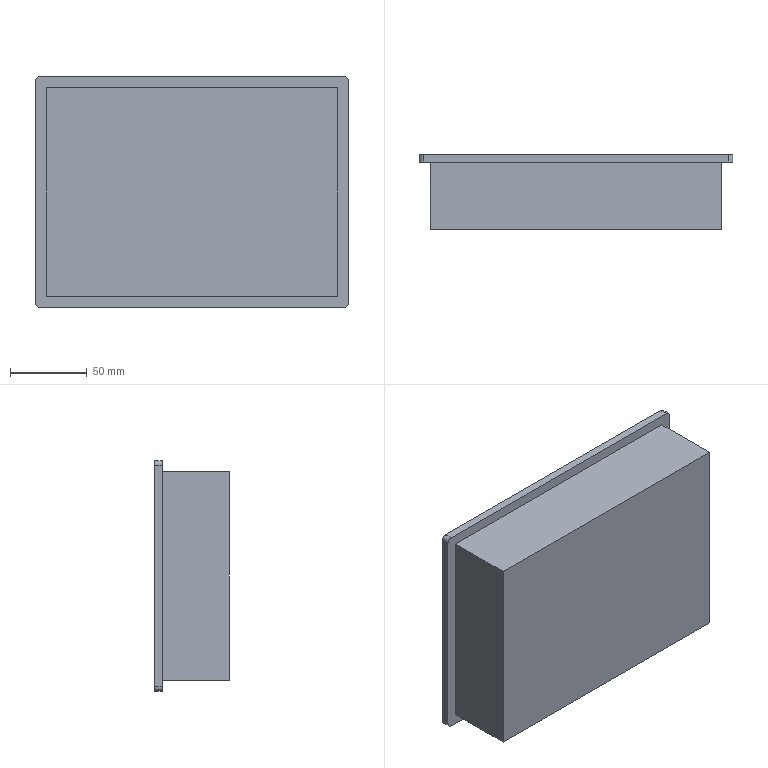Part | STEP file | Weinview-MT506MV5 | 1 solid | 984 faces | box 204 x 48.75 x 150 mm | volume 1264781 mm3 | plane 980 | cylinder 4 | commonest cylinder face diameters 6 x4